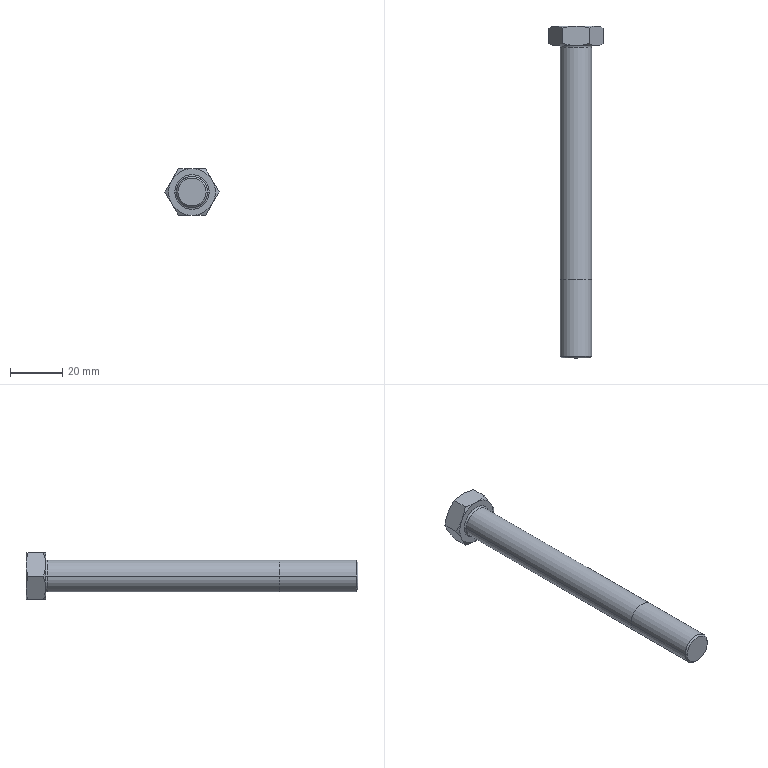Part | NX | features BREP 2 | 1 solid | 31 faces | box 20.785 x 127.5 x 18 mm | volume 16910 mm3 | cone 14 | plane 11 | cylinder 4 | torus 2 | commonest cylinder face diameters 10.106 x2 12 x2